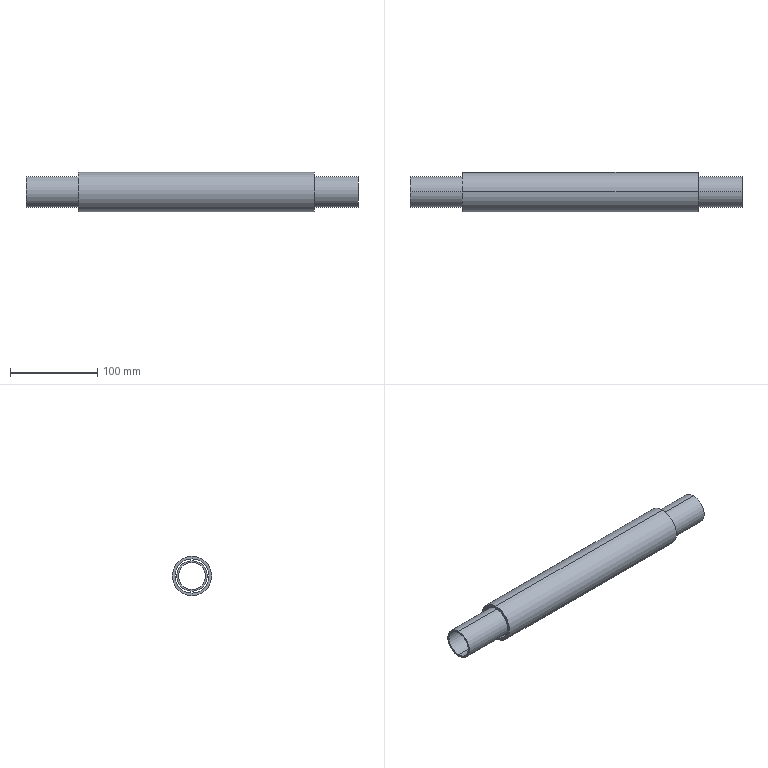Part | STEP file | VIB-C1-3-8-vibration damping pipe 35_default_machined_ | 2 solids | 12 faces | box 380 x 45 x 45 mm | volume 185668 mm3 | cylinder 8 | plane 4 | commonest cylinder face diameters 31 x2 35 x2 39 x2 45 x2
STEP:
#1=CARTESIAN_POINT('',(0.,0.,0.));
#2=DIRECTION('',(0.,0.,1.));
#3=DIRECTION('',(1.,0.,0.));
#4=AXIS2_PLACEMENT_3D('',#1,#2,#3);
#5=CARTESIAN_POINT('',(330.,0.,22.5));
#6=VERTEX_POINT('',#5);
#7=CARTESIAN_POINT('',(330.,0.,-22.5));
#8=VERTEX_POINT('',#7);
#9=CARTESIAN_POINT('',(330.,0.,0.));
#10=DIRECTION('',(-1.,0.,0.));
#11=DIRECTION('',(0.,0.,1.));
#12=AXIS2_PLACEMENT_3D('',#9,#10,#11);
#13=CIRCLE('',#12,22.5);
#14=CARTESIAN_POINT('',(330.,0.,0.));
#15=DIRECTION('',(-1.,0.,0.));
#16=DIRECTION('',(0.,0.,1.));
#17=AXIS2_PLACEMENT_3D('',#14,#15,#16);
#18=CYLINDRICAL_SURFACE('',#17,22.5);
#19=CARTESIAN_POINT('',(0.,0.));
#20=DIRECTION('',(1.,0.));
#21=VECTOR('',#20,1.);
#22=LINE('',#19,#21);
#23=(GEOMETRIC_REPRESENTATION_CONTEXT(2)PARAMETRIC_REPRESENTATION_CONTEXT()REPRESENTATION_CONTEXT('',''));
#24=DEFINITIONAL_REPRESENTATION('',(#22),#23);
#25=PCURVE('',#18,#24);
#26=CARTESIAN_POINT('',(330.,0.,0.));
#27=DIRECTION('',(1.,0.,0.));
#28=DIRECTION('',(0.,0.,-1.));
#29=AXIS2_PLACEMENT_3D('',#26,#27,#28);
#30=PLANE('',#29);
#31=CARTESIAN_POINT('',(-22.5,0.));
#32=CARTESIAN_POINT('',(-22.5,38.971));
#33=CARTESIAN_POINT('',(11.25,19.486));
#34=CARTESIAN_POINT('',(45.,0.));
#35=CARTESIAN_POINT('',(11.25,-19.486));
#36=CARTESIAN_POINT('',(-22.5,-38.971));
#37=CARTESIAN_POINT('',(-22.5,0.));
#38=(BOUNDED_CURVE()B_SPLINE_CURVE(2,(#31,#32,#33,#34,#35,#36,#37),.UNSPECIFIED.,.T.,.F.)B_SPLINE_CURVE_WITH_KNOTS((1,2,2,2,2,1),(-2.094,0.,2.094,4.189,6.283,8.378),.UNSPECIFIED.)CURVE()GEOMETRIC_REPRESENTATION_ITEM()RATIONAL_B_SPLINE_CURVE((1.,0.5,1.,0.5,1.,0.5,1.))REPRESENTATION_ITEM(''));
#39=(GEOMETRIC_REPRESENTATION_CONTEXT(2)PARAMETRIC_REPRESENTATION_CONTEXT()REPRESENTATION_CONTEXT('',''));
#40=DEFINITIONAL_REPRESENTATION('',(#38),#39);
#41=PCURVE('',#30,#40);
#42=SURFACE_CURVE('',#13,(#25,#41),.PCURVE_S1.);
#43=EDGE_CURVE('',#6,#8,#42,.T.);
#44=ORIENTED_EDGE('',*,*,#43,.T.);
#45=CARTESIAN_POINT('',(60.,0.,-22.5));
#46=VERTEX_POINT('',#45);
#47=CARTESIAN_POINT('',(330.,0.,-22.5));
#48=DIRECTION('',(-1.,0.,0.));
#49=VECTOR('',#48,1.);
#50=LINE('',#47,#49);
#51=CARTESIAN_POINT('',(3.142,0.));
#52=DIRECTION('',(0.,1.));
#53=VECTOR('',#52,1.);
#54=LINE('',#51,#53);
#55=(GEOMETRIC_REPRESENTATION_CONTEXT(2)PARAMETRIC_REPRESENTATION_CONTEXT()REPRESENTATION_CONTEXT('',''));
#56=DEFINITIONAL_REPRESENTATION('',(#54),#55);
#57=PCURVE('',#18,#56);
#58=CARTESIAN_POINT('',(330.,0.,0.));
#59=DIRECTION('',(-1.,0.,0.));
#60=DIRECTION('',(0.,0.,1.));
#61=AXIS2_PLACEMENT_3D('',#58,#59,#60);
#62=CYLINDRICAL_SURFACE('',#61,22.5);
#63=CARTESIAN_POINT('',(3.142,0.));
#64=DIRECTION('',(0.,1.));
#65=VECTOR('',#64,1.);
#66=LINE('',#63,#65);
#67=(GEOMETRIC_REPRESENTATION_CONTEXT(2)PARAMETRIC_REPRESENTATION_CONTEXT()REPRESENTATION_CONTEXT('',''));
#68=DEFINITIONAL_REPRESENTATION('',(#66),#67);
#69=PCURVE('',#62,#68);
#70=SURFACE_CURVE('',#50,(#57,#69),.PCURVE_S1.);
#71=EDGE_CURVE('',#8,#46,#70,.T.);
#72=ORIENTED_EDGE('',*,*,#71,.T.);
#73=CARTESIAN_POINT('',(60.,0.,22.5));
#74=VERTEX_POINT('',#73);
#75=CARTESIAN_POINT('',(60.,0.,0.));
#76=DIRECTION('',(1.,0.,0.));
#77=DIRECTION('',(0.,0.,1.));
#78=AXIS2_PLACEMENT_3D('',#75,#76,#77);
#79=CIRCLE('',#78,22.5);
#80=CARTESIAN_POINT('',(6.283,270.));
#81=DIRECTION('',(-1.,0.));
#82=VECTOR('',#81,1.);
#83=LINE('',#80,#82);
#84=(GEOMETRIC_REPRESENTATION_CONTEXT(2)PARAMETRIC_REPRESENTATION_CONTEXT()REPRESENTATION_CONTEXT('',''));
#85=DEFINITIONAL_REPRESENTATION('',(#83),#84);
#86=PCURVE('',#18,#85);
#87=CARTESIAN_POINT('',(60.,0.,0.));
#88=DIRECTION('',(1.,0.,0.));
#89=DIRECTION('',(0.,0.,-1.));
#90=AXIS2_PLACEMENT_3D('',#87,#88,#89);
#91=PLANE('',#90);
#92=CARTESIAN_POINT('',(0.,0.));
#93=DIRECTION('',(-1.,0.));
#94=AXIS2_PLACEMENT_2D('',#92,#93);
#95=CIRCLE('',#94,22.5);
#96=(GEOMETRIC_REPRESENTATION_CONTEXT(2)PARAMETRIC_REPRESENTATION_CONTEXT()REPRESENTATION_CONTEXT('',''));
#97=DEFINITIONAL_REPRESENTATION('',(#95),#96);
#98=PCURVE('',#91,#97);
#99=SURFACE_CURVE('',#79,(#86,#98),.PCURVE_S1.);
#100=EDGE_CURVE('',#46,#74,#99,.T.);
#101=ORIENTED_EDGE('',*,*,#100,.T.);
#102=CARTESIAN_POINT('',(330.,0.,22.5));
#103=DIRECTION('',(-1.,0.,0.));
#104=VECTOR('',#103,1.);
#105=LINE('',#102,#104);
#106=CARTESIAN_POINT('',(0.,0.));
#107=DIRECTION('',(0.,1.));
#108=VECTOR('',#107,1.);
#109=LINE('',#106,#108);
#110=(GEOMETRIC_REPRESENTATION_CONTEXT(2)PARAMETRIC_REPRESENTATION_CONTEXT()REPRESENTATION_CONTEXT('',''));
#111=DEFINITIONAL_REPRESENTATION('',(#109),#110);
#112=PCURVE('',#18,#111);
#113=CARTESIAN_POINT('',(6.283,0.));
#114=DIRECTION('',(0.,1.));
#115=VECTOR('',#114,1.);
#116=LINE('',#113,#115);
#117=(GEOMETRIC_REPRESENTATION_CONTEXT(2)PARAMETRIC_REPRESENTATION_CONTEXT()REPRESENTATION_CONTEXT('',''));
#118=DEFINITIONAL_REPRESENTATION('',(#116),#117);
#119=PCURVE('',#62,#118);
#120=SURFACE_CURVE('',#105,(#112,#119),.PCURVE_S1.);
#121=EDGE_CURVE('',#6,#74,#120,.T.);
#122=ORIENTED_EDGE('',*,*,#121,.F.);
#123=EDGE_LOOP('',(#44,#72,#101,#122));
#124=FACE_BOUND('',#123,.T.);
#125=ADVANCED_FACE('',(#124),#18,.T.);
#126=CARTESIAN_POINT('',(330.,0.,19.5));
#127=VERTEX_POINT('',#126);
#128=CARTESIAN_POINT('',(60.,0.,19.5));
#129=VERTEX_POINT('',#128);
#130=CARTESIAN_POINT('',(330.,0.,19.5));
#131=DIRECTION('',(-1.,0.,0.));
#132=VECTOR('',#131,1.);
#133=LINE('',#130,#132);
#134=CARTESIAN_POINT('',(330.,0.,0.));
#135=DIRECTION('',(-1.,0.,0.));
#136=DIRECTION('',(0.,0.,1.));
#137=AXIS2_PLACEMENT_3D('',#134,#135,#136);
#138=CYLINDRICAL_SURFACE('',#137,19.5);
#139=CARTESIAN_POINT('',(6.283,0.));
#140=DIRECTION('',(0.,1.));
#141=VECTOR('',#140,1.);
#142=LINE('',#139,#141);
#143=(GEOMETRIC_REPRESENTATION_CONTEXT(2)PARAMETRIC_REPRESENTATION_CONTEXT()REPRESENTATION_CONTEXT('',''));
#144=DEFINITIONAL_REPRESENTATION('',(#142),#143);
#145=PCURVE('',#138,#144);
#146=CARTESIAN_POINT('',(330.,0.,0.));
#147=DIRECTION('',(-1.,0.,0.));
#148=DIRECTION('',(0.,0.,1.));
#149=AXIS2_PLACEMENT_3D('',#146,#147,#148);
#150=CYLINDRICAL_SURFACE('',#149,19.5);
#151=CARTESIAN_POINT('',(0.,0.));
#152=DIRECTION('',(0.,1.));
#153=VECTOR('',#152,1.);
#154=LINE('',#151,#153);
#155=(GEOMETRIC_REPRESENTATION_CONTEXT(2)PARAMETRIC_REPRESENTATION_CONTEXT()REPRESENTATION_CONTEXT('',''));
#156=DEFINITIONAL_REPRESENTATION('',(#154),#155);
#157=PCURVE('',#150,#156);
#158=SURFACE_CURVE('',#133,(#145,#157),.PCURVE_S1.);
#159=EDGE_CURVE('',#127,#129,#158,.T.);
#160=ORIENTED_EDGE('',*,*,#159,.T.);
#161=CARTESIAN_POINT('',(60.,0.,-19.5));
#162=VERTEX_POINT('',#161);
#163=CARTESIAN_POINT('',(60.,0.,0.));
#164=DIRECTION('',(-1.,0.,0.));
#165=DIRECTION('',(0.,0.,1.));
#166=AXIS2_PLACEMENT_3D('',#163,#164,#165);
#167=CIRCLE('',#166,19.5);
#168=CARTESIAN_POINT('',(0.,270.));
#169=DIRECTION('',(1.,0.));
#170=VECTOR('',#169,1.);
#171=LINE('',#168,#170);
#172=(GEOMETRIC_REPRESENTATION_CONTEXT(2)PARAMETRIC_REPRESENTATION_CONTEXT()REPRESENTATION_CONTEXT('',''));
#173=DEFINITIONAL_REPRESENTATION('',(#171),#172);
#174=PCURVE('',#138,#173);
#175=CARTESIAN_POINT('',(-19.5,0.));
#176=CARTESIAN_POINT('',(-19.5,33.775));
#177=CARTESIAN_POINT('',(9.75,16.887));
#178=CARTESIAN_POINT('',(39.,0.));
#179=CARTESIAN_POINT('',(9.75,-16.887));
#180=CARTESIAN_POINT('',(-19.5,-33.775));
#181=CARTESIAN_POINT('',(-19.5,0.));
#182=(BOUNDED_CURVE()B_SPLINE_CURVE(2,(#175,#176,#177,#178,#179,#180,#181),.UNSPECIFIED.,.T.,.F.)B_SPLINE_CURVE_WITH_KNOTS((1,2,2,2,2,1),(-2.094,0.,2.094,4.189,6.283,8.378),.UNSPECIFIED.)CURVE()GEOMETRIC_REPRESENTATION_ITEM()RATIONAL_B_SPLINE_CURVE((1.,0.5,1.,0.5,1.,0.5,1.))REPRESENTATION_ITEM(''));
#183=(GEOMETRIC_REPRESENTATION_CONTEXT(2)PARAMETRIC_REPRESENTATION_CONTEXT()REPRESENTATION_CONTEXT('',''));
#184=DEFINITIONAL_REPRESENTATION('',(#182),#183);
#185=PCURVE('',#91,#184);
#186=SURFACE_CURVE('',#167,(#174,#185),.PCURVE_S1.);
#187=EDGE_CURVE('',#162,#129,#186,.T.);
#188=ORIENTED_EDGE('',*,*,#187,.F.);
#189=CARTESIAN_POINT('',(330.,0.,-19.5));
#190=VERTEX_POINT('',#189);
#191=CARTESIAN_POINT('',(330.,0.,-19.5));
#192=DIRECTION('',(-1.,0.,0.));
#193=VECTOR('',#192,1.);
#194=LINE('',#191,#193);
#195=CARTESIAN_POINT('',(3.142,0.));
#196=DIRECTION('',(0.,1.));
#197=VECTOR('',#196,1.);
#198=LINE('',#195,#197);
#199=(GEOMETRIC_REPRESENTATION_CONTEXT(2)PARAMETRIC_REPRESENTATION_CONTEXT()REPRESENTATION_CONTEXT('',''));
#200=DEFINITIONAL_REPRESENTATION('',(#198),#199);
#201=PCURVE('',#138,#200);
#202=CARTESIAN_POINT('',(3.142,0.));
#203=DIRECTION('',(0.,1.));
#204=VECTOR('',#203,1.);
#205=LINE('',#202,#204);
#206=(GEOMETRIC_REPRESENTATION_CONTEXT(2)PARAMETRIC_REPRESENTATION_CONTEXT()REPRESENTATION_CONTEXT('',''));
#207=DEFINITIONAL_REPRESENTATION('',(#205),#206);
#208=PCURVE('',#150,#207);
#209=SURFACE_CURVE('',#194,(#201,#208),.PCURVE_S1.);
#210=EDGE_CURVE('',#190,#162,#209,.T.);
#211=ORIENTED_EDGE('',*,*,#210,.F.);
#212=CARTESIAN_POINT('',(330.,0.,0.));
#213=DIRECTION('',(-1.,0.,0.));
#214=DIRECTION('',(0.,0.,1.));
#215=AXIS2_PLACEMENT_3D('',#212,#213,#214);
#216=CIRCLE('',#215,19.5);
#217=CARTESIAN_POINT('',(0.,0.));
#218=DIRECTION('',(1.,0.));
#219=VECTOR('',#218,1.);
#220=LINE('',#217,#219);
#221=(GEOMETRIC_REPRESENTATION_CONTEXT(2)PARAMETRIC_REPRESENTATION_CONTEXT()REPRESENTATION_CONTEXT('',''));
#222=DEFINITIONAL_REPRESENTATION('',(#220),#221);
#223=PCURVE('',#138,#222);
#224=CARTESIAN_POINT('',(-19.5,0.));
#225=CARTESIAN_POINT('',(-19.5,33.775));
#226=CARTESIAN_POINT('',(9.75,16.887));
#227=CARTESIAN_POINT('',(39.,0.));
#228=CARTESIAN_POINT('',(9.75,-16.887));
#229=CARTESIAN_POINT('',(-19.5,-33.775));
#230=CARTESIAN_POINT('',(-19.5,0.));
#231=(BOUNDED_CURVE()B_SPLINE_CURVE(2,(#224,#225,#226,#227,#228,#229,#230),.UNSPECIFIED.,.T.,.F.)B_SPLINE_CURVE_WITH_KNOTS((1,2,2,2,2,1),(-2.094,0.,2.094,4.189,6.283,8.378),.UNSPECIFIED.)CURVE()GEOMETRIC_REPRESENTATION_ITEM()RATIONAL_B_SPLINE_CURVE((1.,0.5,1.,0.5,1.,0.5,1.))REPRESENTATION_ITEM(''));
#232=(GEOMETRIC_REPRESENTATION_CONTEXT(2)PARAMETRIC_REPRESENTATION_CONTEXT()REPRESENTATION_CONTEXT('',''));
#233=DEFINITIONAL_REPRESENTATION('',(#231),#232);
#234=PCURVE('',#30,#233);
#235=SURFACE_CURVE('',#216,(#223,#234),.PCURVE_S1.);
#236=EDGE_CURVE('',#190,#127,#235,.T.);
#237=ORIENTED_EDGE('',*,*,#236,.T.);
#238=EDGE_LOOP('',(#160,#188,#211,#237));
#239=FACE_BOUND('',#238,.F.);
#240=ADVANCED_FACE('',(#239),#138,.F.);
#241=ORIENTED_EDGE('',*,*,#71,.F.);
#242=CARTESIAN_POINT('',(330.,0.,0.));
#243=DIRECTION('',(-1.,0.,0.));
#244=DIRECTION('',(0.,0.,1.));
#245=AXIS2_PLACEMENT_3D('',#242,#243,#244);
#246=CIRCLE('',#245,22.5);
#247=CARTESIAN_POINT('',(0.,0.));
#248=DIRECTION('',(1.,0.));
#249=VECTOR('',#248,1.);
#250=LINE('',#247,#249);
#251=(GEOMETRIC_REPRESENTATION_CONTEXT(2)PARAMETRIC_REPRESENTATION_CONTEXT()REPRESENTATION_CONTEXT('',''));
#252=DEFINITIONAL_REPRESENTATION('',(#250),#251);
#253=PCURVE('',#62,#252);
#254=CARTESIAN_POINT('',(-22.5,0.));
#255=CARTESIAN_POINT('',(-22.5,38.971));
#256=CARTESIAN_POINT('',(11.25,19.486));
#257=CARTESIAN_POINT('',(45.,0.));
#258=CARTESIAN_POINT('',(11.25,-19.486));
#259=CARTESIAN_POINT('',(-22.5,-38.971));
#260=CARTESIAN_POINT('',(-22.5,0.));
#261=(BOUNDED_CURVE()B_SPLINE_CURVE(2,(#254,#255,#256,#257,#258,#259,#260),.UNSPECIFIED.,.T.,.F.)B_SPLINE_CURVE_WITH_KNOTS((1,2,2,2,2,1),(-2.094,0.,2.094,4.189,6.283,8.378),.UNSPECIFIED.)CURVE()GEOMETRIC_REPRESENTATION_ITEM()RATIONAL_B_SPLINE_CURVE((1.,0.5,1.,0.5,1.,0.5,1.))REPRESENTATION_ITEM(''));
#262=(GEOMETRIC_REPRESENTATION_CONTEXT(2)PARAMETRIC_REPRESENTATION_CONTEXT()REPRESENTATION_CONTEXT('',''));
#263=DEFINITIONAL_REPRESENTATION('',(#261),#262);
#264=PCURVE('',#30,#263);
#265=SURFACE_CURVE('',#246,(#253,#264),.PCURVE_S1.);
#266=EDGE_CURVE('',#8,#6,#265,.T.);
#267=ORIENTED_EDGE('',*,*,#266,.T.);
#268=ORIENTED_EDGE('',*,*,#121,.T.);
#269=CARTESIAN_POINT('',(60.,0.,0.));
#270=DIRECTION('',(1.,0.,0.));
#271=DIRECTION('',(0.,0.,1.));
#272=AXIS2_PLACEMENT_3D('',#269,#270,#271);
#273=CIRCLE('',#272,22.5);
#274=CARTESIAN_POINT('',(6.283,270.));
#275=DIRECTION('',(-1.,0.));
#276=VECTOR('',#275,1.);
#277=LINE('',#274,#276);
#278=(GEOMETRIC_REPRESENTATION_CONTEXT(2)PARAMETRIC_REPRESENTATION_CONTEXT()REPRESENTATION_CONTEXT('',''));
#279=DEFINITIONAL_REPRESENTATION('',(#277),#278);
#280=PCURVE('',#62,#279);
#281=CARTESIAN_POINT('',(0.,0.));
#282=DIRECTION('',(-1.,0.));
#283=AXIS2_PLACEMENT_2D('',#281,#282);
#284=CIRCLE('',#283,22.5);
#285=(GEOMETRIC_REPRESENTATION_CONTEXT(2)PARAMETRIC_REPRESENTATION_CONTEXT()REPRESENTATION_CONTEXT('',''));
#286=DEFINITIONAL_REPRESENTATION('',(#284),#285);
#287=PCURVE('',#91,#286);
#288=SURFACE_CURVE('',#273,(#280,#287),.PCURVE_S1.);
#289=EDGE_CURVE('',#74,#46,#288,.T.);
#290=ORIENTED_EDGE('',*,*,#289,.T.);
#291=EDGE_LOOP('',(#241,#267,#268,#290));
#292=FACE_BOUND('',#291,.T.);
#293=ADVANCED_FACE('',(#292),#62,.T.);
#294=ORIENTED_EDGE('',*,*,#289,.F.);
#295=ORIENTED_EDGE('',*,*,#100,.F.);
#296=EDGE_LOOP('',(#294,#295));
#297=FACE_BOUND('',#296,.T.);
#298=CARTESIAN_POINT('',(60.,0.,0.));
#299=DIRECTION('',(-1.,0.,0.));
#300=DIRECTION('',(0.,0.,1.));
#301=AXIS2_PLACEMENT_3D('',#298,#299,#300);
#302=CIRCLE('',#301,19.5);
#303=CARTESIAN_POINT('',(-19.5,0.));
#304=CARTESIAN_POINT('',(-19.5,33.775));
#305=CARTESIAN_POINT('',(9.75,16.887));
#306=CARTESIAN_POINT('',(39.,0.));
#307=CARTESIAN_POINT('',(9.75,-16.887));
#308=CARTESIAN_POINT('',(-19.5,-33.775));
#309=CARTESIAN_POINT('',(-19.5,0.));
#310=(BOUNDED_CURVE()B_SPLINE_CURVE(2,(#303,#304,#305,#306,#307,#308,#309),.UNSPECIFIED.,.T.,.F.)B_SPLINE_CURVE_WITH_KNOTS((1,2,2,2,2,1),(-2.094,0.,2.094,4.189,6.283,8.378),.UNSPECIFIED.)CURVE()GEOMETRIC_REPRESENTATION_ITEM()RATIONAL_B_SPLINE_CURVE((1.,0.5,1.,0.5,1.,0.5,1.))REPRESENTATION_ITEM(''));
#311=(GEOMETRIC_REPRESENTATION_CONTEXT(2)PARAMETRIC_REPRESENTATION_CONTEXT()REPRESENTATION_CONTEXT('',''));
#312=DEFINITIONAL_REPRESENTATION('',(#310),#311);
#313=PCURVE('',#91,#312);
#314=CARTESIAN_POINT('',(0.,270.));
#315=DIRECTION('',(1.,0.));
#316=VECTOR('',#315,1.);
#317=LINE('',#314,#316);
#318=(GEOMETRIC_REPRESENTATION_CONTEXT(2)PARAMETRIC_REPRESENTATION_CONTEXT()REPRESENTATION_CONTEXT('',''));
#319=DEFINITIONAL_REPRESENTATION('',(#317),#318);
#320=PCURVE('',#150,#319);
#321=SURFACE_CURVE('',#302,(#313,#320),.PCURVE_S1.);
#322=EDGE_CURVE('',#129,#162,#321,.T.);
#323=ORIENTED_EDGE('',*,*,#322,.F.);
#324=ORIENTED_EDGE('',*,*,#187,.F.);
#325=EDGE_LOOP('',(#323,#324));
#326=FACE_BOUND('',#325,.T.);
#327=ADVANCED_FACE('',(#297,#326),#91,.F.);
#328=ORIENTED_EDGE('',*,*,#43,.F.);
#329=ORIENTED_EDGE('',*,*,#266,.F.);
#330=EDGE_LOOP('',(#328,#329));
#331=FACE_BOUND('',#330,.T.);
#332=CARTESIAN_POINT('',(330.,0.,0.));
#333=DIRECTION('',(-1.,0.,0.));
#334=DIRECTION('',(0.,0.,1.));
#335=AXIS2_PLACEMENT_3D('',#332,#333,#334);
#336=CIRCLE('',#335,19.5);
#337=CARTESIAN_POINT('',(-19.5,0.));
#338=CARTESIAN_POINT('',(-19.5,33.775));
#339=CARTESIAN_POINT('',(9.75,16.887));
#340=CARTESIAN_POINT('',(39.,0.));
#341=CARTESIAN_POINT('',(9.75,-16.887));
#342=CARTESIAN_POINT('',(-19.5,-33.775));
#343=CARTESIAN_POINT('',(-19.5,0.));
#344=(BOUNDED_CURVE()B_SPLINE_CURVE(2,(#337,#338,#339,#340,#341,#342,#343),.UNSPECIFIED.,.T.,.F.)B_SPLINE_CURVE_WITH_KNOTS((1,2,2,2,2,1),(-2.094,0.,2.094,4.189,6.283,8.378),.UNSPECIFIED.)CURVE()GEOMETRIC_REPRESENTATION_ITEM()RATIONAL_B_SPLINE_CURVE((1.,0.5,1.,0.5,1.,0.5,1.))REPRESENTATION_ITEM(''));
#345=(GEOMETRIC_REPRESENTATION_CONTEXT(2)PARAMETRIC_REPRESENTATION_CONTEXT()REPRESENTATION_CONTEXT('',''));
#346=DEFINITIONAL_REPRESENTATION('',(#344),#345);
#347=PCURVE('',#30,#346);
#348=CARTESIAN_POINT('',(0.,0.));
#349=DIRECTION('',(1.,0.));
#350=VECTOR('',#349,1.);
#351=LINE('',#348,#350);
#352=(GEOMETRIC_REPRESENTATION_CONTEXT(2)PARAMETRIC_REPRESENTATION_CONTEXT()REPRESENTATION_CONTEXT('',''));
#353=DEFINITIONAL_REPRESENTATION('',(#351),#352);
#354=PCURVE('',#150,#353);
#355=SURFACE_CURVE('',#336,(#347,#354),.PCURVE_S1.);
#356=EDGE_CURVE('',#127,#190,#355,.T.);
#357=ORIENTED_EDGE('',*,*,#356,.T.);
#358=ORIENTED_EDGE('',*,*,#236,.T.);
#359=EDGE_LOOP('',(#357,#358));
#360=FACE_BOUND('',#359,.T.);
#361=ADVANCED_FACE('',(#331,#360),#30,.T.);
#362=ORIENTED_EDGE('',*,*,#322,.F.);
#363=ORIENTED_EDGE('',*,*,#159,.F.);
#364=ORIENTED_EDGE('',*,*,#356,.T.);
#365=ORIENTED_EDGE('',*,*,#210,.T.);
#366=EDGE_LOOP('',(#362,#363,#364,#365));
#367=FACE_BOUND('',#366,.F.);
#368=ADVANCED_FACE('',(#367),#150,.F.);
#369=CLOSED_SHELL('',(#125,#240,#293,#327,#361,#368));
#370=MANIFOLD_SOLID_BREP('',#369);
#371=CARTESIAN_POINT('',(380.,0.,17.5));
#372=VERTEX_POINT('',#371);
#373=CARTESIAN_POINT('',(380.,0.,-17.5));
#374=VERTEX_POINT('',#373);
#375=CARTESIAN_POINT('',(380.,0.,0.));
#376=DIRECTION('',(-1.,0.,0.));
#377=DIRECTION('',(0.,0.,1.));
#378=AXIS2_PLACEMENT_3D('',#375,#376,#377);
#379=CIRCLE('',#378,17.5);
#380=CARTESIAN_POINT('',(380.,0.,0.));
#381=DIRECTION('',(-1.,0.,0.));
#382=DIRECTION('',(0.,0.,1.));
#383=AXIS2_PLACEMENT_3D('',#380,#381,#382);
#384=CYLINDRICAL_SURFACE('',#383,17.5);
#385=CARTESIAN_POINT('',(0.,0.));
#386=DIRECTION('',(1.,0.));
#387=VECTOR('',#386,1.);
#388=LINE('',#385,#387);
#389=(GEOMETRIC_REPRESENTATION_CONTEXT(2)PARAMETRIC_REPRESENTATION_CONTEXT()REPRESENTATION_CONTEXT('',''));
#390=DEFINITIONAL_REPRESENTATION('',(#388),#389);
#391=PCURVE('',#384,#390);
#392=CARTESIAN_POINT('',(380.,0.,0.));
#393=DIRECTION('',(1.,0.,0.));
#394=DIRECTION('',(0.,0.,-1.));
#395=AXIS2_PLACEMENT_3D('',#392,#393,#394);
#396=PLANE('',#395);
#397=CARTESIAN_POINT('',(-17.5,0.));
#398=CARTESIAN_POINT('',(-17.5,30.311));
#399=CARTESIAN_POINT('',(8.75,15.155));
#400=CARTESIAN_POINT('',(35.,0.));
#401=CARTESIAN_POINT('',(8.75,-15.155));
#402=CARTESIAN_POINT('',(-17.5,-30.311));
#403=CARTESIAN_POINT('',(-17.5,0.));
#404=(BOUNDED_CURVE()B_SPLINE_CURVE(2,(#397,#398,#399,#400,#401,#402,#403),.UNSPECIFIED.,.T.,.F.)B_SPLINE_CURVE_WITH_KNOTS((1,2,2,2,2,1),(-2.094,0.,2.094,4.189,6.283,8.378),.UNSPECIFIED.)CURVE()GEOMETRIC_REPRESENTATION_ITEM()RATIONAL_B_SPLINE_CURVE((1.,0.5,1.,0.5,1.,0.5,1.))REPRESENTATION_ITEM(''));
#405=(GEOMETRIC_REPRESENTATION_CONTEXT(2)PARAMETRIC_REPRESENTATION_CONTEXT()REPRESENTATION_CONTEXT('',''));
#406=DEFINITIONAL_REPRESENTATION('',(#404),#405);
#407=PCURVE('',#396,#406);
#408=SURFACE_CURVE('',#379,(#391,#407),.PCURVE_S1.);
#409=EDGE_CURVE('',#372,#374,#408,.T.);
#410=ORIENTED_EDGE('',*,*,#409,.T.);
#411=CARTESIAN_POINT('',(0.,0.,-17.5));
#412=VERTEX_POINT('',#411);
#413=CARTESIAN_POINT('',(380.,0.,-17.5));
#414=DIRECTION('',(-1.,0.,0.));
#415=VECTOR('',#414,1.);
#416=LINE('',#413,#415);
#417=CARTESIAN_POINT('',(3.142,0.));
#418=DIRECTION('',(0.,1.));
#419=VECTOR('',#418,1.);
#420=LINE('',#417,#419);
#421=(GEOMETRIC_REPRESENTATION_CONTEXT(2)PARAMETRIC_REPRESENTATION_CONTEXT()REPRESENTATION_CONTEXT('',''));
#422=DEFINITIONAL_REPRESENTATION('',(#420),#421);
#423=PCURVE('',#384,#422);
#424=CARTESIAN_POINT('',(380.,0.,0.));
#425=DIRECTION('',(-1.,0.,0.));
#426=DIRECTION('',(0.,0.,1.));
#427=AXIS2_PLACEMENT_3D('',#424,#425,#426);
#428=CYLINDRICAL_SURFACE('',#427,17.5);
#429=CARTESIAN_POINT('',(3.142,0.));
#430=DIRECTION('',(0.,1.));
#431=VECTOR('',#430,1.);
#432=LINE('',#429,#431);
#433=(GEOMETRIC_REPRESENTATION_CONTEXT(2)PARAMETRIC_REPRESENTATION_CONTEXT()REPRESENTATION_CONTEXT('',''));
#434=DEFINITIONAL_REPRESENTATION('',(#432),#433);
#435=PCURVE('',#428,#434);
#436=SURFACE_CURVE('',#416,(#423,#435),.PCURVE_S1.);
#437=EDGE_CURVE('',#374,#412,#436,.T.);
#438=ORIENTED_EDGE('',*,*,#437,.T.);
#439=CARTESIAN_POINT('',(0.,0.,17.5));
#440=VERTEX_POINT('',#439);
#441=CARTESIAN_POINT('',(0.,0.,0.));
#442=DIRECTION('',(1.,0.,0.));
#443=DIRECTION('',(0.,0.,1.));
#444=AXIS2_PLACEMENT_3D('',#441,#442,#443);
#445=CIRCLE('',#444,17.5);
#446=CARTESIAN_POINT('',(6.283,380.));
#447=DIRECTION('',(-1.,0.));
#448=VECTOR('',#447,1.);
#449=LINE('',#446,#448);
#450=(GEOMETRIC_REPRESENTATION_CONTEXT(2)PARAMETRIC_REPRESENTATION_CONTEXT()REPRESENTATION_CONTEXT('',''));
#451=DEFINITIONAL_REPRESENTATION('',(#449),#450);
#452=PCURVE('',#384,#451);
#453=CARTESIAN_POINT('',(0.,0.,0.));
#454=DIRECTION('',(1.,0.,0.));
#455=DIRECTION('',(0.,0.,-1.));
#456=AXIS2_PLACEMENT_3D('',#453,#454,#455);
#457=PLANE('',#456);
#458=CARTESIAN_POINT('',(0.,0.));
#459=DIRECTION('',(-1.,0.));
#460=AXIS2_PLACEMENT_2D('',#458,#459);
#461=CIRCLE('',#460,17.5);
#462=(GEOMETRIC_REPRESENTATION_CONTEXT(2)PARAMETRIC_REPRESENTATION_CONTEXT()REPRESENTATION_CONTEXT('',''));
#463=DEFINITIONAL_REPRESENTATION('',(#461),#462);
#464=PCURVE('',#457,#463);
#465=SURFACE_CURVE('',#445,(#452,#464),.PCURVE_S1.);
#466=EDGE_CURVE('',#412,#440,#465,.T.);
#467=ORIENTED_EDGE('',*,*,#466,.T.);
#468=CARTESIAN_POINT('',(380.,0.,17.5));
#469=DIRECTION('',(-1.,0.,0.));
#470=VECTOR('',#469,1.);
#471=LINE('',#468,#470);
#472=CARTESIAN_POINT('',(0.,0.));
#473=DIRECTION('',(0.,1.));
#474=VECTOR('',#473,1.);
#475=LINE('',#472,#474);
#476=(GEOMETRIC_REPRESENTATION_CONTEXT(2)PARAMETRIC_REPRESENTATION_CONTEXT()REPRESENTATION_CONTEXT('',''));
#477=DEFINITIONAL_REPRESENTATION('',(#475),#476);
#478=PCURVE('',#384,#477);
#479=CARTESIAN_POINT('',(6.283,0.));
#480=DIRECTION('',(0.,1.));
#481=VECTOR('',#480,1.);
#482=LINE('',#479,#481);
#483=(GEOMETRIC_REPRESENTATION_CONTEXT(2)PARAMETRIC_REPRESENTATION_CONTEXT()REPRESENTATION_CONTEXT('',''));
#484=DEFINITIONAL_REPRESENTATION('',(#482),#483);
#485=PCURVE('',#428,#484);
#486=SURFACE_CURVE('',#471,(#478,#485),.PCURVE_S1.);
#487=EDGE_CURVE('',#372,#440,#486,.T.);
#488=ORIENTED_EDGE('',*,*,#487,.F.);
#489=EDGE_LOOP('',(#410,#438,#467,#488));
#490=FACE_BOUND('',#489,.T.);
#491=ADVANCED_FACE('',(#490),#384,.T.);
#492=CARTESIAN_POINT('',(380.,0.,15.5));
#493=VERTEX_POINT('',#492);
#494=CARTESIAN_POINT('',(0.,0.,15.5));
#495=VERTEX_POINT('',#494);
#496=CARTESIAN_POINT('',(380.,0.,15.5));
#497=DIRECTION('',(-1.,0.,0.));
#498=VECTOR('',#497,1.);
#499=LINE('',#496,#498);
#500=CARTESIAN_POINT('',(380.,0.,0.));
#501=DIRECTION('',(-1.,0.,0.));
#502=DIRECTION('',(0.,0.,1.));
#503=AXIS2_PLACEMENT_3D('',#500,#501,#502);
#504=CYLINDRICAL_SURFACE('',#503,15.5);
#505=CARTESIAN_POINT('',(6.283,0.));
#506=DIRECTION('',(0.,1.));
#507=VECTOR('',#506,1.);
#508=LINE('',#505,#507);
#509=(GEOMETRIC_REPRESENTATION_CONTEXT(2)PARAMETRIC_REPRESENTATION_CONTEXT()REPRESENTATION_CONTEXT('',''));
#510=DEFINITIONAL_REPRESENTATION('',(#508),#509);
#511=PCURVE('',#504,#510);
#512=CARTESIAN_POINT('',(380.,0.,0.));
#513=DIRECTION('',(-1.,0.,0.));
#514=DIRECTION('',(0.,0.,1.));
#515=AXIS2_PLACEMENT_3D('',#512,#513,#514);
#516=CYLINDRICAL_SURFACE('',#515,15.5);
#517=CARTESIAN_POINT('',(0.,0.));
#518=DIRECTION('',(0.,1.));
#519=VECTOR('',#518,1.);
#520=LINE('',#517,#519);
#521=(GEOMETRIC_REPRESENTATION_CONTEXT(2)PARAMETRIC_REPRESENTATION_CONTEXT()REPRESENTATION_CONTEXT('',''));
#522=DEFINITIONAL_REPRESENTATION('',(#520),#521);
#523=PCURVE('',#516,#522);
#524=SURFACE_CURVE('',#499,(#511,#523),.PCURVE_S1.);
#525=EDGE_CURVE('',#493,#495,#524,.T.);
#526=ORIENTED_EDGE('',*,*,#525,.T.);
#527=CARTESIAN_POINT('',(0.,0.,-15.5));
#528=VERTEX_POINT('',#527);
#529=CARTESIAN_POINT('',(0.,0.,0.));
#530=DIRECTION('',(-1.,0.,0.));
#531=DIRECTION('',(0.,0.,1.));
#532=AXIS2_PLACEMENT_3D('',#529,#530,#531);
#533=CIRCLE('',#532,15.5);
#534=CARTESIAN_POINT('',(0.,380.));
#535=DIRECTION('',(1.,0.));
#536=VECTOR('',#535,1.);
#537=LINE('',#534,#536);
#538=(GEOMETRIC_REPRESENTATION_CONTEXT(2)PARAMETRIC_REPRESENTATION_CONTEXT()REPRESENTATION_CONTEXT('',''));
#539=DEFINITIONAL_REPRESENTATION('',(#537),#538);
#540=PCURVE('',#504,#539);
#541=CARTESIAN_POINT('',(-15.5,0.));
#542=CARTESIAN_POINT('',(-15.5,26.847));
#543=CARTESIAN_POINT('',(7.75,13.423));
#544=CARTESIAN_POINT('',(31.,0.));
#545=CARTESIAN_POINT('',(7.75,-13.423));
#546=CARTESIAN_POINT('',(-15.5,-26.847));
#547=CARTESIAN_POINT('',(-15.5,0.));
#548=(BOUNDED_CURVE()B_SPLINE_CURVE(2,(#541,#542,#543,#544,#545,#546,#547),.UNSPECIFIED.,.T.,.F.)B_SPLINE_CURVE_WITH_KNOTS((1,2,2,2,2,1),(-2.094,0.,2.094,4.189,6.283,8.378),.UNSPECIFIED.)CURVE()GEOMETRIC_REPRESENTATION_ITEM()RATIONAL_B_SPLINE_CURVE((1.,0.5,1.,0.5,1.,0.5,1.))REPRESENTATION_ITEM(''));
#549=(GEOMETRIC_REPRESENTATION_CONTEXT(2)PARAMETRIC_REPRESENTATION_CONTEXT()REPRESENTATION_CONTEXT('',''));
#550=DEFINITIONAL_REPRESENTATION('',(#548),#549);
#551=PCURVE('',#457,#550);
#552=SURFACE_CURVE('',#533,(#540,#551),.PCURVE_S1.);
#553=EDGE_CURVE('',#528,#495,#552,.T.);
#554=ORIENTED_EDGE('',*,*,#553,.F.);
#555=CARTESIAN_POINT('',(380.,0.,-15.5));
#556=VERTEX_POINT('',#555);
#557=CARTESIAN_POINT('',(380.,0.,-15.5));
#558=DIRECTION('',(-1.,0.,0.));
#559=VECTOR('',#558,1.);
#560=LINE('',#557,#559);
#561=CARTESIAN_POINT('',(3.142,0.));
#562=DIRECTION('',(0.,1.));
#563=VECTOR('',#562,1.);
#564=LINE('',#561,#563);
#565=(GEOMETRIC_REPRESENTATION_CONTEXT(2)PARAMETRIC_REPRESENTATION_CONTEXT()REPRESENTATION_CONTEXT('',''));
#566=DEFINITIONAL_REPRESENTATION('',(#564),#565);
#567=PCURVE('',#504,#566);
#568=CARTESIAN_POINT('',(3.142,0.));
#569=DIRECTION('',(0.,1.));
#570=VECTOR('',#569,1.);
#571=LINE('',#568,#570);
#572=(GEOMETRIC_REPRESENTATION_CONTEXT(2)PARAMETRIC_REPRESENTATION_CONTEXT()REPRESENTATION_CONTEXT('',''));
#573=DEFINITIONAL_REPRESENTATION('',(#571),#572);
#574=PCURVE('',#516,#573);
#575=SURFACE_CURVE('',#560,(#567,#574),.PCURVE_S1.);
#576=EDGE_CURVE('',#556,#528,#575,.T.);
#577=ORIENTED_EDGE('',*,*,#576,.F.);
#578=CARTESIAN_POINT('',(380.,0.,0.));
#579=DIRECTION('',(-1.,0.,0.));
#580=DIRECTION('',(0.,0.,1.));
#581=AXIS2_PLACEMENT_3D('',#578,#579,#580);
#582=CIRCLE('',#581,15.5);
#583=CARTESIAN_POINT('',(0.,0.));
#584=DIRECTION('',(1.,0.));
#585=VECTOR('',#584,1.);
#586=LINE('',#583,#585);
#587=(GEOMETRIC_REPRESENTATION_CONTEXT(2)PARAMETRIC_REPRESENTATION_CONTEXT()REPRESENTATION_CONTEXT('',''));
#588=DEFINITIONAL_REPRESENTATION('',(#586),#587);
#589=PCURVE('',#504,#588);
#590=CARTESIAN_POINT('',(-15.5,0.));
#591=CARTESIAN_POINT('',(-15.5,26.847));
#592=CARTESIAN_POINT('',(7.75,13.423));
#593=CARTESIAN_POINT('',(31.,0.));
#594=CARTESIAN_POINT('',(7.75,-13.423));
#595=CARTESIAN_POINT('',(-15.5,-26.847));
#596=CARTESIAN_POINT('',(-15.5,0.));
#597=(BOUNDED_CURVE()B_SPLINE_CURVE(2,(#590,#591,#592,#593,#594,#595,#596),.UNSPECIFIED.,.T.,.F.)B_SPLINE_CURVE_WITH_KNOTS((1,2,2,2,2,1),(-2.094,0.,2.094,4.189,6.283,8.378),.UNSPECIFIED.)CURVE()GEOMETRIC_REPRESENTATION_ITEM()RATIONAL_B_SPLINE_CURVE((1.,0.5,1.,0.5,1.,0.5,1.))REPRESENTATION_ITEM(''));
#598=(GEOMETRIC_REPRESENTATION_CONTEXT(2)PARAMETRIC_REPRESENTATION_CONTEXT()REPRESENTATION_CONTEXT('',''));
#599=DEFINITIONAL_REPRESENTATION('',(#597),#598);
#600=PCURVE('',#396,#599);
#601=SURFACE_CURVE('',#582,(#589,#600),.PCURVE_S1.);
#602=EDGE_CURVE('',#556,#493,#601,.T.);
#603=ORIENTED_EDGE('',*,*,#602,.T.);
#604=EDGE_LOOP('',(#526,#554,#577,#603));
#605=FACE_BOUND('',#604,.F.);
#606=ADVANCED_FACE('',(#605),#504,.F.);
#607=ORIENTED_EDGE('',*,*,#437,.F.);
#608=CARTESIAN_POINT('',(380.,0.,0.));
#609=DIRECTION('',(-1.,0.,0.));
#610=DIRECTION('',(0.,0.,1.));
#611=AXIS2_PLACEMENT_3D('',#608,#609,#610);
#612=CIRCLE('',#611,17.5);
#613=CARTESIAN_POINT('',(0.,0.));
#614=DIRECTION('',(1.,0.));
#615=VECTOR('',#614,1.);
#616=LINE('',#613,#615);
#617=(GEOMETRIC_REPRESENTATION_CONTEXT(2)PARAMETRIC_REPRESENTATION_CONTEXT()REPRESENTATION_CONTEXT('',''));
#618=DEFINITIONAL_REPRESENTATION('',(#616),#617);
#619=PCURVE('',#428,#618);
#620=CARTESIAN_POINT('',(-17.5,0.));
#621=CARTESIAN_POINT('',(-17.5,30.311));
#622=CARTESIAN_POINT('',(8.75,15.155));
#623=CARTESIAN_POINT('',(35.,0.));
#624=CARTESIAN_POINT('',(8.75,-15.155));
#625=CARTESIAN_POINT('',(-17.5,-30.311));
#626=CARTESIAN_POINT('',(-17.5,0.));
#627=(BOUNDED_CURVE()B_SPLINE_CURVE(2,(#620,#621,#622,#623,#624,#625,#626),.UNSPECIFIED.,.T.,.F.)B_SPLINE_CURVE_WITH_KNOTS((1,2,2,2,2,1),(-2.094,0.,2.094,4.189,6.283,8.378),.UNSPECIFIED.)CURVE()GEOMETRIC_REPRESENTATION_ITEM()RATIONAL_B_SPLINE_CURVE((1.,0.5,1.,0.5,1.,0.5,1.))REPRESENTATION_ITEM(''));
#628=(GEOMETRIC_REPRESENTATION_CONTEXT(2)PARAMETRIC_REPRESENTATION_CONTEXT()REPRESENTATION_CONTEXT('',''));
#629=DEFINITIONAL_REPRESENTATION('',(#627),#628);
#630=PCURVE('',#396,#629);
#631=SURFACE_CURVE('',#612,(#619,#630),.PCURVE_S1.);
#632=EDGE_CURVE('',#374,#372,#631,.T.);
#633=ORIENTED_EDGE('',*,*,#632,.T.);
#634=ORIENTED_EDGE('',*,*,#487,.T.);
#635=CARTESIAN_POINT('',(0.,0.,0.));
#636=DIRECTION('',(1.,0.,0.));
#637=DIRECTION('',(0.,0.,1.));
#638=AXIS2_PLACEMENT_3D('',#635,#636,#637);
#639=CIRCLE('',#638,17.5);
#640=CARTESIAN_POINT('',(6.283,380.));
#641=DIRECTION('',(-1.,0.));
#642=VECTOR('',#641,1.);
#643=LINE('',#640,#642);
#644=(GEOMETRIC_REPRESENTATION_CONTEXT(2)PARAMETRIC_REPRESENTATION_CONTEXT()REPRESENTATION_CONTEXT('',''));
#645=DEFINITIONAL_REPRESENTATION('',(#643),#644);
#646=PCURVE('',#428,#645);
#647=CARTESIAN_POINT('',(0.,0.));
#648=DIRECTION('',(-1.,0.));
#649=AXIS2_PLACEMENT_2D('',#647,#648);
#650=CIRCLE('',#649,17.5);
#651=(GEOMETRIC_REPRESENTATION_CONTEXT(2)PARAMETRIC_REPRESENTATION_CONTEXT()REPRESENTATION_CONTEXT('',''));
#652=DEFINITIONAL_REPRESENTATION('',(#650),#651);
#653=PCURVE('',#457,#652);
#654=SURFACE_CURVE('',#639,(#646,#653),.PCURVE_S1.);
#655=EDGE_CURVE('',#440,#412,#654,.T.);
#656=ORIENTED_EDGE('',*,*,#655,.T.);
#657=EDGE_LOOP('',(#607,#633,#634,#656));
#658=FACE_BOUND('',#657,.T.);
#659=ADVANCED_FACE('',(#658),#428,.T.);
#660=ORIENTED_EDGE('',*,*,#655,.F.);
#661=ORIENTED_EDGE('',*,*,#466,.F.);
#662=EDGE_LOOP('',(#660,#661));
#663=FACE_BOUND('',#662,.T.);
#664=CARTESIAN_POINT('',(0.,0.,0.));
#665=DIRECTION('',(-1.,0.,0.));
#666=DIRECTION('',(0.,0.,1.));
#667=AXIS2_PLACEMENT_3D('',#664,#665,#666);
#668=CIRCLE('',#667,15.5);
#669=CARTESIAN_POINT('',(-15.5,0.));
#670=CARTESIAN_POINT('',(-15.5,26.847));
#671=CARTESIAN_POINT('',(7.75,13.423));
#672=CARTESIAN_POINT('',(31.,0.));
#673=CARTESIAN_POINT('',(7.75,-13.423));
#674=CARTESIAN_POINT('',(-15.5,-26.847));
#675=CARTESIAN_POINT('',(-15.5,0.));
#676=(BOUNDED_CURVE()B_SPLINE_CURVE(2,(#669,#670,#671,#672,#673,#674,#675),.UNSPECIFIED.,.T.,.F.)B_SPLINE_CURVE_WITH_KNOTS((1,2,2,2,2,1),(-2.094,0.,2.094,4.189,6.283,8.378),.UNSPECIFIED.)CURVE()GEOMETRIC_REPRESENTATION_ITEM()RATIONAL_B_SPLINE_CURVE((1.,0.5,1.,0.5,1.,0.5,1.))REPRESENTATION_ITEM(''));
#677=(GEOMETRIC_REPRESENTATION_CONTEXT(2)PARAMETRIC_REPRESENTATION_CONTEXT()REPRESENTATION_CONTEXT('',''));
#678=DEFINITIONAL_REPRESENTATION('',(#676),#677);
#679=PCURVE('',#457,#678);
#680=CARTESIAN_POINT('',(0.,380.));
#681=DIRECTION('',(1.,0.));
#682=VECTOR('',#681,1.);
#683=LINE('',#680,#682);
#684=(GEOMETRIC_REPRESENTATION_CONTEXT(2)PARAMETRIC_REPRESENTATION_CONTEXT()REPRESENTATION_CONTEXT('',''));
#685=DEFINITIONAL_REPRESENTATION('',(#683),#684);
#686=PCURVE('',#516,#685);
#687=SURFACE_CURVE('',#668,(#679,#686),.PCURVE_S1.);
#688=EDGE_CURVE('',#495,#528,#687,.T.);
#689=ORIENTED_EDGE('',*,*,#688,.F.);
#690=ORIENTED_EDGE('',*,*,#553,.F.);
#691=EDGE_LOOP('',(#689,#690));
#692=FACE_BOUND('',#691,.T.);
#693=ADVANCED_FACE('',(#663,#692),#457,.F.);
#694=ORIENTED_EDGE('',*,*,#409,.F.);
#695=ORIENTED_EDGE('',*,*,#632,.F.);
#696=EDGE_LOOP('',(#694,#695));
#697=FACE_BOUND('',#696,.T.);
#698=CARTESIAN_POINT('',(380.,0.,0.));
#699=DIRECTION('',(-1.,0.,0.));
#700=DIRECTION('',(0.,0.,1.));
#701=AXIS2_PLACEMENT_3D('',#698,#699,#700);
#702=CIRCLE('',#701,15.5);
#703=CARTESIAN_POINT('',(-15.5,0.));
#704=CARTESIAN_POINT('',(-15.5,26.847));
#705=CARTESIAN_POINT('',(7.75,13.423));
#706=CARTESIAN_POINT('',(31.,0.));
#707=CARTESIAN_POINT('',(7.75,-13.423));
#708=CARTESIAN_POINT('',(-15.5,-26.847));
#709=CARTESIAN_POINT('',(-15.5,0.));
#710=(BOUNDED_CURVE()B_SPLINE_CURVE(2,(#703,#704,#705,#706,#707,#708,#709),.UNSPECIFIED.,.T.,.F.)B_SPLINE_CURVE_WITH_KNOTS((1,2,2,2,2,1),(-2.094,0.,2.094,4.189,6.283,8.378),.UNSPECIFIED.)CURVE()GEOMETRIC_REPRESENTATION_ITEM()RATIONAL_B_SPLINE_CURVE((1.,0.5,1.,0.5,1.,0.5,1.))REPRESENTATION_ITEM(''));
#711=(GEOMETRIC_REPRESENTATION_CONTEXT(2)PARAMETRIC_REPRESENTATION_CONTEXT()REPRESENTATION_CONTEXT('',''));
#712=DEFINITIONAL_REPRESENTATION('',(#710),#711);
#713=PCURVE('',#396,#712);
#714=CARTESIAN_POINT('',(0.,0.));
#715=DIRECTION('',(1.,0.));
#716=VECTOR('',#715,1.);
#717=LINE('',#714,#716);
#718=(GEOMETRIC_REPRESENTATION_CONTEXT(2)PARAMETRIC_REPRESENTATION_CONTEXT()REPRESENTATION_CONTEXT('',''));
#719=DEFINITIONAL_REPRESENTATION('',(#717),#718);
#720=PCURVE('',#516,#719);
#721=SURFACE_CURVE('',#702,(#713,#720),.PCURVE_S1.);
#722=EDGE_CURVE('',#493,#556,#721,.T.);
#723=ORIENTED_EDGE('',*,*,#722,.T.);
#724=ORIENTED_EDGE('',*,*,#602,.T.);
#725=EDGE_LOOP('',(#723,#724));
#726=FACE_BOUND('',#725,.T.);
#727=ADVANCED_FACE('',(#697,#726),#396,.T.);
#728=ORIENTED_EDGE('',*,*,#688,.F.);
#729=ORIENTED_EDGE('',*,*,#525,.F.);
#730=ORIENTED_EDGE('',*,*,#722,.T.);
#731=ORIENTED_EDGE('',*,*,#576,.T.);
#732=EDGE_LOOP('',(#728,#729,#730,#731));
#733=FACE_BOUND('',#732,.F.);
#734=ADVANCED_FACE('',(#733),#516,.F.);
#735=CLOSED_SHELL('',(#491,#606,#659,#693,#727,#734));
#736=MANIFOLD_SOLID_BREP('',#735);
#737=(LENGTH_UNIT()NAMED_UNIT(*)SI_UNIT(.MILLI.,.METRE.));
#738=UNCERTAINTY_MEASURE_WITH_UNIT(LENGTH_MEASURE(0.0000001),#737,'','');
#739=(NAMED_UNIT(*)PLANE_ANGLE_UNIT()SI_UNIT($,.RADIAN.));
#740=(NAMED_UNIT(*)SI_UNIT($,.STERADIAN.)SOLID_ANGLE_UNIT());
#741=(GEOMETRIC_REPRESENTATION_CONTEXT(3)GLOBAL_UNCERTAINTY_ASSIGNED_CONTEXT((#738))GLOBAL_UNIT_ASSIGNED_CONTEXT((#737,#739,#740))REPRESENTATION_CONTEXT('',''));
#742=SHAPE_REPRESENTATION('',(#4,#370,#736),#741);